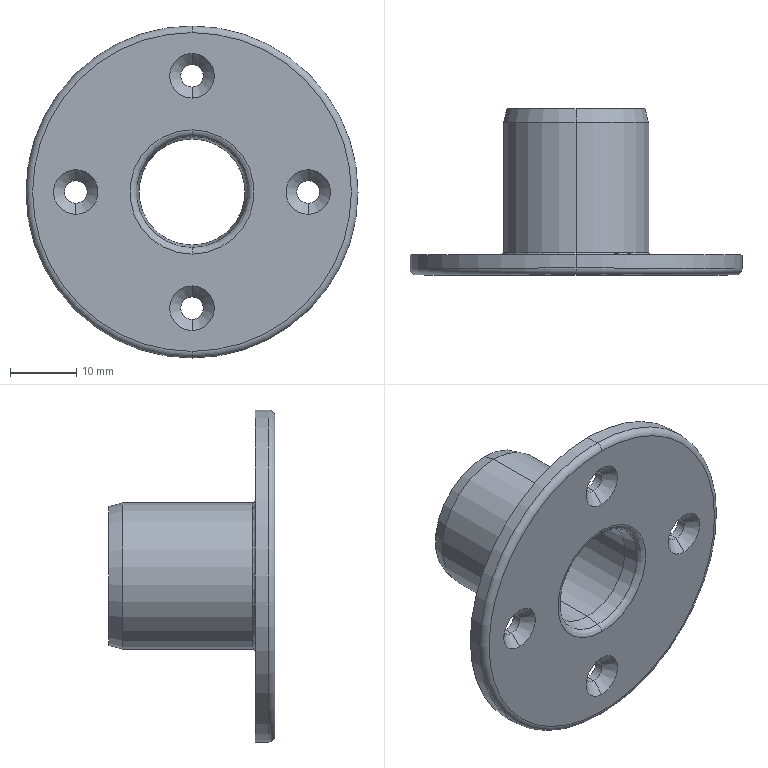Part | STEP file | MPSZ16-12_Default | 1 solid | 39 faces | box 50 x 25 x 50 mm | volume 8876 mm3 | cone 14 | cylinder 14 | torus 8 | plane 3 | commonest cylinder face diameters 3.4 x8 16 x2 22 x2 50 x2